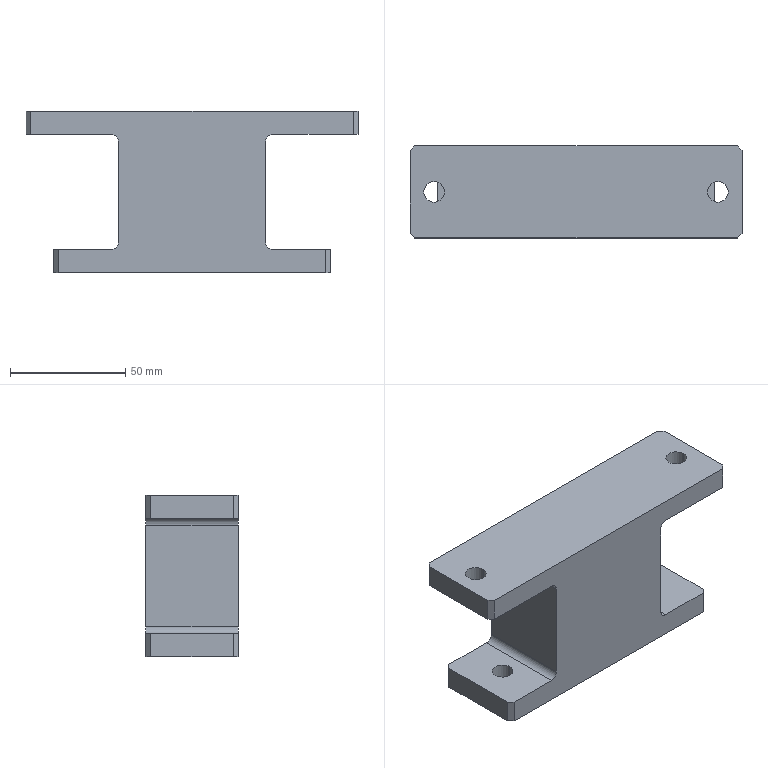Part | SolidWorks | features ICE 4, 3DProfileFeature 3, HoleWzd 3, Cut 2, Chamfer 1, Extrusion 1, Fillet 1, MirrorPattern 1 | 1 solid | 34 faces | box 144 x 40 x 70 mm | volume 231204 mm3 | plane 22 | cylinder 12 | commonest cylinder face diameters 9 x8 6 x4
STEP:
#1=CARTESIAN_POINT('',(78.784,24.549,10.));
#2=VERTEX_POINT('',#1);
#3=CARTESIAN_POINT('',(69.784,24.549,10.));
#4=VERTEX_POINT('',#3);
#5=CARTESIAN_POINT('',(74.284,24.549,10.));
#6=DIRECTION('',(0.,0.,-1.));
#7=DIRECTION('',(-1.,0.,0.));
#8=AXIS2_PLACEMENT_3D('',#5,#6,#7);
#9=CIRCLE('',#8,4.5);
#10=EDGE_CURVE('',#2,#4,#9,.T.);
#11=ORIENTED_EDGE('',*,*,#10,.F.);
#12=CARTESIAN_POINT('',(78.784,24.549,0.));
#13=VERTEX_POINT('',#12);
#14=CARTESIAN_POINT('',(78.784,24.549,0.));
#15=DIRECTION('',(0.,0.,-1.));
#16=VECTOR('',#15,1000.);
#17=LINE('',#14,#16);
#18=EDGE_CURVE('',#2,#13,#17,.T.);
#19=ORIENTED_EDGE('',*,*,#18,.T.);
#20=CARTESIAN_POINT('',(69.784,24.549,0.));
#21=VERTEX_POINT('',#20);
#22=CARTESIAN_POINT('',(74.284,24.549,0.));
#23=DIRECTION('',(0.,0.,-1.));
#24=DIRECTION('',(-1.,0.,0.));
#25=AXIS2_PLACEMENT_3D('',#22,#23,#24);
#26=CIRCLE('',#25,4.5);
#27=EDGE_CURVE('',#13,#21,#26,.T.);
#28=ORIENTED_EDGE('',*,*,#27,.T.);
#29=CARTESIAN_POINT('',(69.784,24.549,0.));
#30=DIRECTION('',(0.,0.,-1.));
#31=VECTOR('',#30,1000.);
#32=LINE('',#29,#31);
#33=EDGE_CURVE('',#4,#21,#32,.T.);
#34=ORIENTED_EDGE('',*,*,#33,.F.);
#35=EDGE_LOOP('',(#11,#19,#28,#34));
#36=FACE_OUTER_BOUND('',#35,.T.);
#37=CARTESIAN_POINT('',(74.284,24.549,0.));
#38=DIRECTION('',(0.,0.,-1.));
#39=DIRECTION('',(-1.,0.,0.));
#40=AXIS2_PLACEMENT_3D('',#37,#38,#39);
#41=CYLINDRICAL_SURFACE('',#40,4.5);
#42=ADVANCED_FACE('',(#36),#41,.F.);
#43=CARTESIAN_POINT('',(168.784,24.549,10.));
#44=VERTEX_POINT('',#43);
#45=CARTESIAN_POINT('',(159.784,24.549,10.));
#46=VERTEX_POINT('',#45);
#47=CARTESIAN_POINT('',(164.284,24.549,10.));
#48=DIRECTION('',(0.,0.,-1.));
#49=DIRECTION('',(-1.,0.,0.));
#50=AXIS2_PLACEMENT_3D('',#47,#48,#49);
#51=CIRCLE('',#50,4.5);
#52=EDGE_CURVE('',#44,#46,#51,.T.);
#53=ORIENTED_EDGE('',*,*,#52,.F.);
#54=CARTESIAN_POINT('',(168.784,24.549,0.));
#55=VERTEX_POINT('',#54);
#56=CARTESIAN_POINT('',(168.784,24.549,0.));
#57=DIRECTION('',(0.,0.,-1.));
#58=VECTOR('',#57,1000.);
#59=LINE('',#56,#58);
#60=EDGE_CURVE('',#44,#55,#59,.T.);
#61=ORIENTED_EDGE('',*,*,#60,.T.);
#62=CARTESIAN_POINT('',(159.784,24.549,0.));
#63=VERTEX_POINT('',#62);
#64=CARTESIAN_POINT('',(164.284,24.549,0.));
#65=DIRECTION('',(0.,0.,-1.));
#66=DIRECTION('',(-1.,0.,0.));
#67=AXIS2_PLACEMENT_3D('',#64,#65,#66);
#68=CIRCLE('',#67,4.5);
#69=EDGE_CURVE('',#55,#63,#68,.T.);
#70=ORIENTED_EDGE('',*,*,#69,.T.);
#71=CARTESIAN_POINT('',(159.784,24.549,0.));
#72=DIRECTION('',(0.,0.,-1.));
#73=VECTOR('',#72,1000.);
#74=LINE('',#71,#73);
#75=EDGE_CURVE('',#46,#63,#74,.T.);
#76=ORIENTED_EDGE('',*,*,#75,.F.);
#77=EDGE_LOOP('',(#53,#61,#70,#76));
#78=FACE_OUTER_BOUND('',#77,.T.);
#79=CARTESIAN_POINT('',(164.284,24.549,0.));
#80=DIRECTION('',(0.,0.,-1.));
#81=DIRECTION('',(-1.,0.,0.));
#82=AXIS2_PLACEMENT_3D('',#79,#80,#81);
#83=CYLINDRICAL_SURFACE('',#82,4.5);
#84=ADVANCED_FACE('',(#78),#83,.F.);
#85=CARTESIAN_POINT('',(176.284,24.549,60.));
#86=VERTEX_POINT('',#85);
#87=CARTESIAN_POINT('',(185.284,24.549,60.));
#88=VERTEX_POINT('',#87);
#89=CARTESIAN_POINT('',(180.784,24.549,60.));
#90=DIRECTION('',(0.,0.,1.));
#91=DIRECTION('',(1.,0.,0.));
#92=AXIS2_PLACEMENT_3D('',#89,#90,#91);
#93=CIRCLE('',#92,4.5);
#94=EDGE_CURVE('',#86,#88,#93,.T.);
#95=ORIENTED_EDGE('',*,*,#94,.F.);
#96=CARTESIAN_POINT('',(176.284,24.549,70.));
#97=VERTEX_POINT('',#96);
#98=CARTESIAN_POINT('',(176.284,24.549,47.272));
#99=DIRECTION('',(0.,0.,1.));
#100=VECTOR('',#99,1000.);
#101=LINE('',#98,#100);
#102=EDGE_CURVE('',#86,#97,#101,.T.);
#103=ORIENTED_EDGE('',*,*,#102,.T.);
#104=CARTESIAN_POINT('',(185.284,24.549,70.));
#105=VERTEX_POINT('',#104);
#106=CARTESIAN_POINT('',(180.784,24.549,70.));
#107=DIRECTION('',(0.,0.,-1.));
#108=DIRECTION('',(-1.,0.,0.));
#109=AXIS2_PLACEMENT_3D('',#106,#107,#108);
#110=CIRCLE('',#109,4.5);
#111=EDGE_CURVE('',#105,#97,#110,.T.);
#112=ORIENTED_EDGE('',*,*,#111,.F.);
#113=CARTESIAN_POINT('',(185.284,24.549,47.272));
#114=DIRECTION('',(0.,0.,1.));
#115=VECTOR('',#114,1000.);
#116=LINE('',#113,#115);
#117=EDGE_CURVE('',#88,#105,#116,.T.);
#118=ORIENTED_EDGE('',*,*,#117,.F.);
#119=EDGE_LOOP('',(#95,#103,#112,#118));
#120=FACE_OUTER_BOUND('',#119,.T.);
#121=CARTESIAN_POINT('',(180.784,24.549,47.272));
#122=DIRECTION('',(0.,0.,1.));
#123=DIRECTION('',(1.,0.,0.));
#124=AXIS2_PLACEMENT_3D('',#121,#122,#123);
#125=CYLINDRICAL_SURFACE('',#124,4.5);
#126=ADVANCED_FACE('',(#120),#125,.F.);
#127=CARTESIAN_POINT('',(62.284,24.549,60.));
#128=VERTEX_POINT('',#127);
#129=CARTESIAN_POINT('',(53.284,24.549,60.));
#130=VERTEX_POINT('',#129);
#131=CARTESIAN_POINT('',(57.784,24.549,60.));
#132=DIRECTION('',(0.,0.,-1.));
#133=DIRECTION('',(1.,0.,0.));
#134=AXIS2_PLACEMENT_3D('',#131,#132,#133);
#135=CIRCLE('',#134,4.5);
#136=EDGE_CURVE('',#128,#130,#135,.T.);
#137=ORIENTED_EDGE('',*,*,#136,.T.);
#138=CARTESIAN_POINT('',(53.284,24.549,70.));
#139=VERTEX_POINT('',#138);
#140=CARTESIAN_POINT('',(53.284,24.549,47.272));
#141=DIRECTION('',(0.,0.,1.));
#142=VECTOR('',#141,1000.);
#143=LINE('',#140,#142);
#144=EDGE_CURVE('',#130,#139,#143,.T.);
#145=ORIENTED_EDGE('',*,*,#144,.T.);
#146=CARTESIAN_POINT('',(62.284,24.549,70.));
#147=VERTEX_POINT('',#146);
#148=CARTESIAN_POINT('',(57.784,24.549,70.));
#149=DIRECTION('',(0.,0.,1.));
#150=DIRECTION('',(1.,0.,0.));
#151=AXIS2_PLACEMENT_3D('',#148,#149,#150);
#152=CIRCLE('',#151,4.5);
#153=EDGE_CURVE('',#139,#147,#152,.T.);
#154=ORIENTED_EDGE('',*,*,#153,.T.);
#155=CARTESIAN_POINT('',(62.284,24.549,47.272));
#156=DIRECTION('',(0.,0.,1.));
#157=VECTOR('',#156,1000.);
#158=LINE('',#155,#157);
#159=EDGE_CURVE('',#128,#147,#158,.T.);
#160=ORIENTED_EDGE('',*,*,#159,.F.);
#161=EDGE_LOOP('',(#137,#145,#154,#160));
#162=FACE_OUTER_BOUND('',#161,.T.);
#163=CARTESIAN_POINT('',(57.784,24.549,47.272));
#164=DIRECTION('',(0.,0.,1.));
#165=DIRECTION('',(1.,0.,0.));
#166=AXIS2_PLACEMENT_3D('',#163,#164,#165);
#167=CYLINDRICAL_SURFACE('',#166,4.5);
#168=ADVANCED_FACE('',(#162),#167,.F.);
#169=CARTESIAN_POINT('',(179.284,6.549,0.));
#170=VERTEX_POINT('',#169);
#171=CARTESIAN_POINT('',(179.284,42.549,0.));
#172=VERTEX_POINT('',#171);
#173=CARTESIAN_POINT('',(179.284,44.549,0.));
#174=DIRECTION('',(0.,1.,0.));
#175=VECTOR('',#174,1000.);
#176=LINE('',#173,#175);
#177=EDGE_CURVE('',#170,#172,#176,.T.);
#178=ORIENTED_EDGE('',*,*,#177,.T.);
#179=CARTESIAN_POINT('',(179.284,42.549,10.));
#180=VERTEX_POINT('',#179);
#181=CARTESIAN_POINT('',(179.284,42.549,70.));
#182=DIRECTION('',(0.,0.,1.));
#183=VECTOR('',#182,1000.);
#184=LINE('',#181,#183);
#185=EDGE_CURVE('',#172,#180,#184,.T.);
#186=ORIENTED_EDGE('',*,*,#185,.T.);
#187=CARTESIAN_POINT('',(179.284,6.549,10.));
#188=VERTEX_POINT('',#187);
#189=CARTESIAN_POINT('',(179.284,44.549,10.));
#190=DIRECTION('',(0.,-1.,0.));
#191=VECTOR('',#190,1000.);
#192=LINE('',#189,#191);
#193=EDGE_CURVE('',#180,#188,#192,.T.);
#194=ORIENTED_EDGE('',*,*,#193,.T.);
#195=CARTESIAN_POINT('',(179.284,6.549,70.));
#196=DIRECTION('',(0.,0.,-1.));
#197=VECTOR('',#196,1000.);
#198=LINE('',#195,#197);
#199=EDGE_CURVE('',#188,#170,#198,.T.);
#200=ORIENTED_EDGE('',*,*,#199,.T.);
#201=EDGE_LOOP('',(#178,#186,#194,#200));
#202=FACE_OUTER_BOUND('',#201,.T.);
#203=CARTESIAN_POINT('',(179.284,44.549,70.));
#204=DIRECTION('',(-1.,0.,0.));
#205=DIRECTION('',(0.,0.,1.));
#206=AXIS2_PLACEMENT_3D('',#203,#204,#205);
#207=PLANE('',#206);
#208=ADVANCED_FACE('',(#202),#207,.F.);
#209=CARTESIAN_POINT('',(177.284,44.549,0.));
#210=VERTEX_POINT('',#209);
#211=CARTESIAN_POINT('',(61.284,44.549,0.));
#212=VERTEX_POINT('',#211);
#213=CARTESIAN_POINT('',(179.284,44.549,0.));
#214=DIRECTION('',(-1.,0.,0.));
#215=VECTOR('',#214,1000.);
#216=LINE('',#213,#215);
#217=EDGE_CURVE('',#210,#212,#216,.T.);
#218=ORIENTED_EDGE('',*,*,#217,.T.);
#219=CARTESIAN_POINT('',(61.284,44.549,10.));
#220=VERTEX_POINT('',#219);
#221=CARTESIAN_POINT('',(61.284,44.549,70.));
#222=DIRECTION('',(0.,0.,1.));
#223=VECTOR('',#222,1000.);
#224=LINE('',#221,#223);
#225=EDGE_CURVE('',#212,#220,#224,.T.);
#226=ORIENTED_EDGE('',*,*,#225,.T.);
#227=CARTESIAN_POINT('',(84.284,44.549,10.));
#228=VERTEX_POINT('',#227);
#229=CARTESIAN_POINT('',(87.284,44.549,10.));
#230=DIRECTION('',(-1.,0.,0.));
#231=VECTOR('',#230,1000.);
#232=LINE('',#229,#231);
#233=EDGE_CURVE('',#228,#220,#232,.T.);
#234=ORIENTED_EDGE('',*,*,#233,.F.);
#235=CARTESIAN_POINT('',(87.284,44.549,13.));
#236=VERTEX_POINT('',#235);
#237=CARTESIAN_POINT('',(84.284,44.549,13.));
#238=DIRECTION('',(0.,-1.,0.));
#239=DIRECTION('',(0.,0.,-1.));
#240=AXIS2_PLACEMENT_3D('',#237,#238,#239);
#241=CIRCLE('',#240,3.);
#242=EDGE_CURVE('',#228,#236,#241,.T.);
#243=ORIENTED_EDGE('',*,*,#242,.T.);
#244=CARTESIAN_POINT('',(87.284,44.549,57.));
#245=VERTEX_POINT('',#244);
#246=CARTESIAN_POINT('',(87.284,44.549,60.));
#247=DIRECTION('',(0.,0.,-1.));
#248=VECTOR('',#247,1000.);
#249=LINE('',#246,#248);
#250=EDGE_CURVE('',#245,#236,#249,.T.);
#251=ORIENTED_EDGE('',*,*,#250,.F.);
#252=CARTESIAN_POINT('',(84.284,44.549,60.));
#253=VERTEX_POINT('',#252);
#254=CARTESIAN_POINT('',(84.284,44.549,57.));
#255=DIRECTION('',(0.,-1.,0.));
#256=DIRECTION('',(0.,0.,-1.));
#257=AXIS2_PLACEMENT_3D('',#254,#255,#256);
#258=CIRCLE('',#257,3.);
#259=EDGE_CURVE('',#245,#253,#258,.T.);
#260=ORIENTED_EDGE('',*,*,#259,.T.);
#261=CARTESIAN_POINT('',(49.284,44.549,60.));
#262=VERTEX_POINT('',#261);
#263=CARTESIAN_POINT('',(87.284,44.549,60.));
#264=DIRECTION('',(1.,0.,0.));
#265=VECTOR('',#264,1000.);
#266=LINE('',#263,#265);
#267=EDGE_CURVE('',#262,#253,#266,.T.);
#268=ORIENTED_EDGE('',*,*,#267,.F.);
#269=CARTESIAN_POINT('',(49.284,44.549,70.));
#270=VERTEX_POINT('',#269);
#271=CARTESIAN_POINT('',(49.284,44.549,70.));
#272=DIRECTION('',(0.,0.,1.));
#273=VECTOR('',#272,1000.);
#274=LINE('',#271,#273);
#275=EDGE_CURVE('',#262,#270,#274,.T.);
#276=ORIENTED_EDGE('',*,*,#275,.T.);
#277=CARTESIAN_POINT('',(189.284,44.549,70.));
#278=VERTEX_POINT('',#277);
#279=CARTESIAN_POINT('',(179.284,44.549,70.));
#280=DIRECTION('',(-1.,0.,0.));
#281=VECTOR('',#280,1000.);
#282=LINE('',#279,#281);
#283=EDGE_CURVE('',#278,#270,#282,.T.);
#284=ORIENTED_EDGE('',*,*,#283,.F.);
#285=CARTESIAN_POINT('',(189.284,44.549,60.));
#286=VERTEX_POINT('',#285);
#287=CARTESIAN_POINT('',(189.284,44.549,60.));
#288=DIRECTION('',(0.,0.,-1.));
#289=VECTOR('',#288,1000.);
#290=LINE('',#287,#289);
#291=EDGE_CURVE('',#278,#286,#290,.T.);
#292=ORIENTED_EDGE('',*,*,#291,.T.);
#293=CARTESIAN_POINT('',(154.284,44.549,60.));
#294=VERTEX_POINT('',#293);
#295=CARTESIAN_POINT('',(151.284,44.549,60.));
#296=DIRECTION('',(1.,0.,0.));
#297=VECTOR('',#296,1000.);
#298=LINE('',#295,#297);
#299=EDGE_CURVE('',#294,#286,#298,.T.);
#300=ORIENTED_EDGE('',*,*,#299,.F.);
#301=CARTESIAN_POINT('',(151.284,44.549,57.));
#302=VERTEX_POINT('',#301);
#303=CARTESIAN_POINT('',(154.284,44.549,57.));
#304=DIRECTION('',(0.,-1.,0.));
#305=DIRECTION('',(0.,0.,-1.));
#306=AXIS2_PLACEMENT_3D('',#303,#304,#305);
#307=CIRCLE('',#306,3.);
#308=EDGE_CURVE('',#294,#302,#307,.T.);
#309=ORIENTED_EDGE('',*,*,#308,.T.);
#310=CARTESIAN_POINT('',(151.284,44.549,13.));
#311=VERTEX_POINT('',#310);
#312=CARTESIAN_POINT('',(151.284,44.549,60.));
#313=DIRECTION('',(0.,0.,1.));
#314=VECTOR('',#313,1000.);
#315=LINE('',#312,#314);
#316=EDGE_CURVE('',#311,#302,#315,.T.);
#317=ORIENTED_EDGE('',*,*,#316,.F.);
#318=CARTESIAN_POINT('',(154.284,44.549,10.));
#319=VERTEX_POINT('',#318);
#320=CARTESIAN_POINT('',(154.284,44.549,13.));
#321=DIRECTION('',(0.,-1.,0.));
#322=DIRECTION('',(0.,0.,-1.));
#323=AXIS2_PLACEMENT_3D('',#320,#321,#322);
#324=CIRCLE('',#323,3.);
#325=EDGE_CURVE('',#311,#319,#324,.T.);
#326=ORIENTED_EDGE('',*,*,#325,.T.);
#327=CARTESIAN_POINT('',(177.284,44.549,10.));
#328=VERTEX_POINT('',#327);
#329=CARTESIAN_POINT('',(151.284,44.549,10.));
#330=DIRECTION('',(-1.,0.,0.));
#331=VECTOR('',#330,1000.);
#332=LINE('',#329,#331);
#333=EDGE_CURVE('',#328,#319,#332,.T.);
#334=ORIENTED_EDGE('',*,*,#333,.F.);
#335=CARTESIAN_POINT('',(177.284,44.549,70.));
#336=DIRECTION('',(0.,0.,-1.));
#337=VECTOR('',#336,1000.);
#338=LINE('',#335,#337);
#339=EDGE_CURVE('',#328,#210,#338,.T.);
#340=ORIENTED_EDGE('',*,*,#339,.T.);
#341=EDGE_LOOP('',(#218,#226,#234,#243,#251,#260,#268,#276,#284,#292,#300,#309,#317,#326,#334,#340));
#342=FACE_OUTER_BOUND('',#341,.T.);
#343=CARTESIAN_POINT('',(179.284,44.549,70.));
#344=DIRECTION('',(0.,-1.,0.));
#345=DIRECTION('',(0.,0.,-1.));
#346=AXIS2_PLACEMENT_3D('',#343,#344,#345);
#347=PLANE('',#346);
#348=ADVANCED_FACE('',(#342),#347,.F.);
#349=CARTESIAN_POINT('',(59.284,42.549,0.));
#350=VERTEX_POINT('',#349);
#351=CARTESIAN_POINT('',(59.284,6.549,0.));
#352=VERTEX_POINT('',#351);
#353=CARTESIAN_POINT('',(59.284,44.549,0.));
#354=DIRECTION('',(0.,-1.,0.));
#355=VECTOR('',#354,1000.);
#356=LINE('',#353,#355);
#357=EDGE_CURVE('',#350,#352,#356,.T.);
#358=ORIENTED_EDGE('',*,*,#357,.T.);
#359=CARTESIAN_POINT('',(59.284,6.549,10.));
#360=VERTEX_POINT('',#359);
#361=CARTESIAN_POINT('',(59.284,6.549,70.));
#362=DIRECTION('',(0.,0.,1.));
#363=VECTOR('',#362,1000.);
#364=LINE('',#361,#363);
#365=EDGE_CURVE('',#352,#360,#364,.T.);
#366=ORIENTED_EDGE('',*,*,#365,.T.);
#367=CARTESIAN_POINT('',(59.284,42.549,10.));
#368=VERTEX_POINT('',#367);
#369=CARTESIAN_POINT('',(59.284,44.549,10.));
#370=DIRECTION('',(0.,1.,0.));
#371=VECTOR('',#370,1000.);
#372=LINE('',#369,#371);
#373=EDGE_CURVE('',#360,#368,#372,.T.);
#374=ORIENTED_EDGE('',*,*,#373,.T.);
#375=CARTESIAN_POINT('',(59.284,42.549,70.));
#376=DIRECTION('',(0.,0.,-1.));
#377=VECTOR('',#376,1000.);
#378=LINE('',#375,#377);
#379=EDGE_CURVE('',#368,#350,#378,.T.);
#380=ORIENTED_EDGE('',*,*,#379,.T.);
#381=EDGE_LOOP('',(#358,#366,#374,#380));
#382=FACE_OUTER_BOUND('',#381,.T.);
#383=CARTESIAN_POINT('',(59.284,44.549,70.));
#384=DIRECTION('',(1.,0.,0.));
#385=DIRECTION('',(0.,0.,-1.));
#386=AXIS2_PLACEMENT_3D('',#383,#384,#385);
#387=PLANE('',#386);
#388=ADVANCED_FACE('',(#382),#387,.F.);
#389=CARTESIAN_POINT('',(84.284,4.549,10.));
#390=VERTEX_POINT('',#389);
#391=CARTESIAN_POINT('',(61.284,4.549,10.));
#392=VERTEX_POINT('',#391);
#393=CARTESIAN_POINT('',(87.284,4.549,10.));
#394=DIRECTION('',(-1.,0.,0.));
#395=VECTOR('',#394,1000.);
#396=LINE('',#393,#395);
#397=EDGE_CURVE('',#390,#392,#396,.T.);
#398=ORIENTED_EDGE('',*,*,#397,.T.);
#399=CARTESIAN_POINT('',(61.284,4.549,0.));
#400=VERTEX_POINT('',#399);
#401=CARTESIAN_POINT('',(61.284,4.549,70.));
#402=DIRECTION('',(0.,0.,-1.));
#403=VECTOR('',#402,1000.);
#404=LINE('',#401,#403);
#405=EDGE_CURVE('',#392,#400,#404,.T.);
#406=ORIENTED_EDGE('',*,*,#405,.T.);
#407=CARTESIAN_POINT('',(177.284,4.549,0.));
#408=VERTEX_POINT('',#407);
#409=CARTESIAN_POINT('',(179.284,4.549,0.));
#410=DIRECTION('',(1.,0.,0.));
#411=VECTOR('',#410,1000.);
#412=LINE('',#409,#411);
#413=EDGE_CURVE('',#400,#408,#412,.T.);
#414=ORIENTED_EDGE('',*,*,#413,.T.);
#415=CARTESIAN_POINT('',(177.284,4.549,10.));
#416=VERTEX_POINT('',#415);
#417=CARTESIAN_POINT('',(177.284,4.549,70.));
#418=DIRECTION('',(0.,0.,1.));
#419=VECTOR('',#418,1000.);
#420=LINE('',#417,#419);
#421=EDGE_CURVE('',#408,#416,#420,.T.);
#422=ORIENTED_EDGE('',*,*,#421,.T.);
#423=CARTESIAN_POINT('',(154.284,4.549,10.));
#424=VERTEX_POINT('',#423);
#425=CARTESIAN_POINT('',(151.284,4.549,10.));
#426=DIRECTION('',(-1.,0.,0.));
#427=VECTOR('',#426,1000.);
#428=LINE('',#425,#427);
#429=EDGE_CURVE('',#416,#424,#428,.T.);
#430=ORIENTED_EDGE('',*,*,#429,.T.);
#431=CARTESIAN_POINT('',(151.284,4.549,13.));
#432=VERTEX_POINT('',#431);
#433=CARTESIAN_POINT('',(154.284,4.549,13.));
#434=DIRECTION('',(0.,1.,0.));
#435=DIRECTION('',(-1.,0.,0.));
#436=AXIS2_PLACEMENT_3D('',#433,#434,#435);
#437=CIRCLE('',#436,3.);
#438=EDGE_CURVE('',#424,#432,#437,.T.);
#439=ORIENTED_EDGE('',*,*,#438,.T.);
#440=CARTESIAN_POINT('',(151.284,4.549,57.));
#441=VERTEX_POINT('',#440);
#442=CARTESIAN_POINT('',(151.284,4.549,60.));
#443=DIRECTION('',(0.,0.,1.));
#444=VECTOR('',#443,1000.);
#445=LINE('',#442,#444);
#446=EDGE_CURVE('',#432,#441,#445,.T.);
#447=ORIENTED_EDGE('',*,*,#446,.T.);
#448=CARTESIAN_POINT('',(154.284,4.549,60.));
#449=VERTEX_POINT('',#448);
#450=CARTESIAN_POINT('',(154.284,4.549,57.));
#451=DIRECTION('',(0.,1.,0.));
#452=DIRECTION('',(-1.,0.,0.));
#453=AXIS2_PLACEMENT_3D('',#450,#451,#452);
#454=CIRCLE('',#453,3.);
#455=EDGE_CURVE('',#441,#449,#454,.T.);
#456=ORIENTED_EDGE('',*,*,#455,.T.);
#457=CARTESIAN_POINT('',(189.284,4.549,60.));
#458=VERTEX_POINT('',#457);
#459=CARTESIAN_POINT('',(151.284,4.549,60.));
#460=DIRECTION('',(1.,0.,0.));
#461=VECTOR('',#460,1000.);
#462=LINE('',#459,#461);
#463=EDGE_CURVE('',#449,#458,#462,.T.);
#464=ORIENTED_EDGE('',*,*,#463,.T.);
#465=CARTESIAN_POINT('',(189.284,4.549,70.));
#466=VERTEX_POINT('',#465);
#467=CARTESIAN_POINT('',(189.284,4.549,70.));
#468=DIRECTION('',(0.,0.,1.));
#469=VECTOR('',#468,1000.);
#470=LINE('',#467,#469);
#471=EDGE_CURVE('',#458,#466,#470,.T.);
#472=ORIENTED_EDGE('',*,*,#471,.T.);
#473=CARTESIAN_POINT('',(49.284,4.549,70.));
#474=VERTEX_POINT('',#473);
#475=CARTESIAN_POINT('',(179.284,4.549,70.));
#476=DIRECTION('',(1.,0.,0.));
#477=VECTOR('',#476,1000.);
#478=LINE('',#475,#477);
#479=EDGE_CURVE('',#474,#466,#478,.T.);
#480=ORIENTED_EDGE('',*,*,#479,.F.);
#481=CARTESIAN_POINT('',(49.284,4.549,60.));
#482=VERTEX_POINT('',#481);
#483=CARTESIAN_POINT('',(49.284,4.549,60.));
#484=DIRECTION('',(0.,0.,-1.));
#485=VECTOR('',#484,1000.);
#486=LINE('',#483,#485);
#487=EDGE_CURVE('',#474,#482,#486,.T.);
#488=ORIENTED_EDGE('',*,*,#487,.T.);
#489=CARTESIAN_POINT('',(84.284,4.549,60.));
#490=VERTEX_POINT('',#489);
#491=CARTESIAN_POINT('',(87.284,4.549,60.));
#492=DIRECTION('',(1.,0.,0.));
#493=VECTOR('',#492,1000.);
#494=LINE('',#491,#493);
#495=EDGE_CURVE('',#482,#490,#494,.T.);
#496=ORIENTED_EDGE('',*,*,#495,.T.);
#497=CARTESIAN_POINT('',(87.284,4.549,57.));
#498=VERTEX_POINT('',#497);
#499=CARTESIAN_POINT('',(84.284,4.549,57.));
#500=DIRECTION('',(0.,1.,0.));
#501=DIRECTION('',(-1.,0.,0.));
#502=AXIS2_PLACEMENT_3D('',#499,#500,#501);
#503=CIRCLE('',#502,3.);
#504=EDGE_CURVE('',#490,#498,#503,.T.);
#505=ORIENTED_EDGE('',*,*,#504,.T.);
#506=CARTESIAN_POINT('',(87.284,4.549,13.));
#507=VERTEX_POINT('',#506);
#508=CARTESIAN_POINT('',(87.284,4.549,60.));
#509=DIRECTION('',(0.,0.,-1.));
#510=VECTOR('',#509,1000.);
#511=LINE('',#508,#510);
#512=EDGE_CURVE('',#498,#507,#511,.T.);
#513=ORIENTED_EDGE('',*,*,#512,.T.);
#514=CARTESIAN_POINT('',(84.284,4.549,13.));
#515=DIRECTION('',(0.,1.,0.));
#516=DIRECTION('',(-1.,0.,0.));
#517=AXIS2_PLACEMENT_3D('',#514,#515,#516);
#518=CIRCLE('',#517,3.);
#519=EDGE_CURVE('',#507,#390,#518,.T.);
#520=ORIENTED_EDGE('',*,*,#519,.T.);
#521=EDGE_LOOP('',(#398,#406,#414,#422,#430,#439,#447,#456,#464,#472,#480,#488,#496,#505,#513,#520));
#522=FACE_OUTER_BOUND('',#521,.T.);
#523=CARTESIAN_POINT('',(179.284,4.549,70.));
#524=DIRECTION('',(0.,1.,0.));
#525=DIRECTION('',(-1.,0.,0.));
#526=AXIS2_PLACEMENT_3D('',#523,#524,#525);
#527=PLANE('',#526);
#528=ADVANCED_FACE('',(#522),#527,.F.);
#529=ORIENTED_EDGE('',*,*,#111,.T.);
#530=CARTESIAN_POINT('',(180.784,24.549,70.));
#531=DIRECTION('',(0.,0.,-1.));
#532=DIRECTION('',(-1.,0.,0.));
#533=AXIS2_PLACEMENT_3D('',#530,#531,#532);
#534=CIRCLE('',#533,4.5);
#535=EDGE_CURVE('',#97,#105,#534,.T.);
#536=ORIENTED_EDGE('',*,*,#535,.T.);
#537=EDGE_LOOP('',(#529,#536));
#538=FACE_BOUND('',#537,.T.);
#539=CARTESIAN_POINT('',(57.784,24.549,70.));
#540=DIRECTION('',(0.,0.,1.));
#541=DIRECTION('',(1.,0.,0.));
#542=AXIS2_PLACEMENT_3D('',#539,#540,#541);
#543=CIRCLE('',#542,4.5);
#544=EDGE_CURVE('',#147,#139,#543,.T.);
#545=ORIENTED_EDGE('',*,*,#544,.F.);
#546=ORIENTED_EDGE('',*,*,#153,.F.);
#547=EDGE_LOOP('',(#545,#546));
#548=FACE_BOUND('',#547,.T.);
#549=ORIENTED_EDGE('',*,*,#479,.T.);
#550=CARTESIAN_POINT('',(191.284,6.549,70.));
#551=VERTEX_POINT('',#550);
#552=CARTESIAN_POINT('',(191.284,6.549,70.));
#553=DIRECTION('',(0.7071,0.7071,0.));
#554=VECTOR('',#553,1000.);
#555=LINE('',#552,#554);
#556=EDGE_CURVE('',#466,#551,#555,.T.);
#557=ORIENTED_EDGE('',*,*,#556,.T.);
#558=CARTESIAN_POINT('',(191.284,42.549,70.));
#559=VERTEX_POINT('',#558);
#560=CARTESIAN_POINT('',(191.284,4.549,70.));
#561=DIRECTION('',(0.,-1.,0.));
#562=VECTOR('',#561,1000.);
#563=LINE('',#560,#562);
#564=EDGE_CURVE('',#559,#551,#563,.T.);
#565=ORIENTED_EDGE('',*,*,#564,.F.);
#566=CARTESIAN_POINT('',(189.284,44.549,70.));
#567=DIRECTION('',(-0.7071,0.7071,0.));
#568=VECTOR('',#567,1000.);
#569=LINE('',#566,#568);
#570=EDGE_CURVE('',#559,#278,#569,.T.);
#571=ORIENTED_EDGE('',*,*,#570,.T.);
#572=ORIENTED_EDGE('',*,*,#283,.T.);
#573=CARTESIAN_POINT('',(47.284,42.549,70.));
#574=VERTEX_POINT('',#573);
#575=CARTESIAN_POINT('',(49.284,44.549,70.));
#576=DIRECTION('',(-0.7071,-0.7071,0.));
#577=VECTOR('',#576,1000.);
#578=LINE('',#575,#577);
#579=EDGE_CURVE('',#270,#574,#578,.T.);
#580=ORIENTED_EDGE('',*,*,#579,.T.);
#581=CARTESIAN_POINT('',(47.284,6.549,70.));
#582=VERTEX_POINT('',#581);
#583=CARTESIAN_POINT('',(47.284,44.549,70.));
#584=DIRECTION('',(0.,-1.,0.));
#585=VECTOR('',#584,1000.);
#586=LINE('',#583,#585);
#587=EDGE_CURVE('',#574,#582,#586,.T.);
#588=ORIENTED_EDGE('',*,*,#587,.T.);
#589=CARTESIAN_POINT('',(47.284,6.549,70.));
#590=DIRECTION('',(0.7071,-0.7071,0.));
#591=VECTOR('',#590,1000.);
#592=LINE('',#589,#591);
#593=EDGE_CURVE('',#582,#474,#592,.T.);
#594=ORIENTED_EDGE('',*,*,#593,.T.);
#595=EDGE_LOOP('',(#549,#557,#565,#571,#572,#580,#588,#594));
#596=FACE_OUTER_BOUND('',#595,.T.);
#597=CARTESIAN_POINT('',(0.,0.,70.));
#598=DIRECTION('',(0.,0.,-1.));
#599=DIRECTION('',(-1.,0.,0.));
#600=AXIS2_PLACEMENT_3D('',#597,#598,#599);
#601=PLANE('',#600);
#602=ADVANCED_FACE('',(#538,#548,#596),#601,.F.);
#603=CARTESIAN_POINT('',(74.284,24.549,0.));
#604=DIRECTION('',(0.,0.,-1.));
#605=DIRECTION('',(-1.,0.,0.));
#606=AXIS2_PLACEMENT_3D('',#603,#604,#605);
#607=CIRCLE('',#606,4.5);
#608=EDGE_CURVE('',#21,#13,#607,.T.);
#609=ORIENTED_EDGE('',*,*,#608,.F.);
#610=ORIENTED_EDGE('',*,*,#27,.F.);
#611=EDGE_LOOP('',(#609,#610));
#612=FACE_BOUND('',#611,.T.);
#613=CARTESIAN_POINT('',(164.284,24.549,0.));
#614=DIRECTION('',(0.,0.,-1.));
#615=DIRECTION('',(-1.,0.,0.));
#616=AXIS2_PLACEMENT_3D('',#613,#614,#615);
#617=CIRCLE('',#616,4.5);
#618=EDGE_CURVE('',#63,#55,#617,.T.);
#619=ORIENTED_EDGE('',*,*,#618,.F.);
#620=ORIENTED_EDGE('',*,*,#69,.F.);
#621=EDGE_LOOP('',(#619,#620));
#622=FACE_BOUND('',#621,.T.);
#623=ORIENTED_EDGE('',*,*,#413,.F.);
#624=CARTESIAN_POINT('',(32.917,32.917,0.));
#625=DIRECTION('',(-0.7071,0.7071,0.));
#626=VECTOR('',#625,1000.);
#627=LINE('',#624,#626);
#628=EDGE_CURVE('',#400,#352,#627,.T.);
#629=ORIENTED_EDGE('',*,*,#628,.T.);
#630=ORIENTED_EDGE('',*,*,#357,.F.);
#631=CARTESIAN_POINT('',(8.368,-8.368,0.));
#632=DIRECTION('',(0.7071,0.7071,0.));
#633=VECTOR('',#632,1000.);
#634=LINE('',#631,#633);
#635=EDGE_CURVE('',#350,#212,#634,.T.);
#636=ORIENTED_EDGE('',*,*,#635,.T.);
#637=ORIENTED_EDGE('',*,*,#217,.F.);
#638=CARTESIAN_POINT('',(110.917,110.917,0.));
#639=DIRECTION('',(0.7071,-0.7071,0.));
#640=VECTOR('',#639,1000.);
#641=LINE('',#638,#640);
#642=EDGE_CURVE('',#210,#172,#641,.T.);
#643=ORIENTED_EDGE('',*,*,#642,.T.);
#644=ORIENTED_EDGE('',*,*,#177,.F.);
#645=CARTESIAN_POINT('',(86.368,-86.368,0.));
#646=DIRECTION('',(-0.7071,-0.7071,0.));
#647=VECTOR('',#646,1000.);
#648=LINE('',#645,#647);
#649=EDGE_CURVE('',#170,#408,#648,.T.);
#650=ORIENTED_EDGE('',*,*,#649,.T.);
#651=EDGE_LOOP('',(#623,#629,#630,#636,#637,#643,#644,#650));
#652=FACE_OUTER_BOUND('',#651,.T.);
#653=CARTESIAN_POINT('',(0.,0.,0.));
#654=DIRECTION('',(0.,0.,-1.));
#655=DIRECTION('',(-1.,0.,0.));
#656=AXIS2_PLACEMENT_3D('',#653,#654,#655);
#657=PLANE('',#656);
#658=ADVANCED_FACE('',(#612,#622,#652),#657,.T.);
#659=CARTESIAN_POINT('',(164.284,24.549,10.));
#660=DIRECTION('',(0.,0.,-1.));
#661=DIRECTION('',(-1.,0.,0.));
#662=AXIS2_PLACEMENT_3D('',#659,#660,#661);
#663=CIRCLE('',#662,4.5);
#664=EDGE_CURVE('',#46,#44,#663,.T.);
#665=ORIENTED_EDGE('',*,*,#664,.T.);
#666=ORIENTED_EDGE('',*,*,#52,.T.);
#667=EDGE_LOOP('',(#665,#666));
#668=FACE_BOUND('',#667,.T.);
#669=ORIENTED_EDGE('',*,*,#193,.F.);
#670=CARTESIAN_POINT('',(177.284,44.549,10.));
#671=DIRECTION('',(-0.7071,0.7071,0.));
#672=VECTOR('',#671,1000.);
#673=LINE('',#670,#672);
#674=EDGE_CURVE('',#180,#328,#673,.T.);
#675=ORIENTED_EDGE('',*,*,#674,.T.);
#676=ORIENTED_EDGE('',*,*,#333,.T.);
#677=CARTESIAN_POINT('',(154.284,4.549,10.));
#678=DIRECTION('',(0.,-1.,0.));
#679=VECTOR('',#678,1000.);
#680=LINE('',#677,#679);
#681=EDGE_CURVE('',#319,#424,#680,.T.);
#682=ORIENTED_EDGE('',*,*,#681,.T.);
#683=ORIENTED_EDGE('',*,*,#429,.F.);
#684=CARTESIAN_POINT('',(179.284,6.549,10.));
#685=DIRECTION('',(0.7071,0.7071,0.));
#686=VECTOR('',#685,1000.);
#687=LINE('',#684,#686);
#688=EDGE_CURVE('',#416,#188,#687,.T.);
#689=ORIENTED_EDGE('',*,*,#688,.T.);
#690=EDGE_LOOP('',(#669,#675,#676,#682,#683,#689));
#691=FACE_OUTER_BOUND('',#690,.T.);
#692=CARTESIAN_POINT('',(151.284,4.549,10.));
#693=DIRECTION('',(0.,0.,-1.));
#694=DIRECTION('',(-1.,0.,0.));
#695=AXIS2_PLACEMENT_3D('',#692,#693,#694);
#696=PLANE('',#695);
#697=ADVANCED_FACE('',(#668,#691),#696,.F.);
#698=CARTESIAN_POINT('',(180.784,24.549,60.));
#699=DIRECTION('',(0.,0.,1.));
#700=DIRECTION('',(1.,0.,0.));
#701=AXIS2_PLACEMENT_3D('',#698,#699,#700);
#702=CIRCLE('',#701,4.5);
#703=EDGE_CURVE('',#88,#86,#702,.T.);
#704=ORIENTED_EDGE('',*,*,#703,.T.);
#705=ORIENTED_EDGE('',*,*,#94,.T.);
#706=EDGE_LOOP('',(#704,#705));
#707=FACE_BOUND('',#706,.T.);
#708=CARTESIAN_POINT('',(191.284,42.549,60.));
#709=VERTEX_POINT('',#708);
#710=CARTESIAN_POINT('',(191.284,6.549,60.));
#711=VERTEX_POINT('',#710);
#712=CARTESIAN_POINT('',(191.284,4.549,60.));
#713=DIRECTION('',(0.,-1.,0.));
#714=VECTOR('',#713,1000.);
#715=LINE('',#712,#714);
#716=EDGE_CURVE('',#709,#711,#715,.T.);
#717=ORIENTED_EDGE('',*,*,#716,.T.);
#718=CARTESIAN_POINT('',(191.284,6.549,60.));
#719=DIRECTION('',(-0.7071,-0.7071,0.));
#720=VECTOR('',#719,1000.);
#721=LINE('',#718,#720);
#722=EDGE_CURVE('',#711,#458,#721,.T.);
#723=ORIENTED_EDGE('',*,*,#722,.T.);
#724=ORIENTED_EDGE('',*,*,#463,.F.);
#725=CARTESIAN_POINT('',(154.284,44.549,60.));
#726=DIRECTION('',(0.,1.,0.));
#727=VECTOR('',#726,1000.);
#728=LINE('',#725,#727);
#729=EDGE_CURVE('',#449,#294,#728,.T.);
#730=ORIENTED_EDGE('',*,*,#729,.T.);
#731=ORIENTED_EDGE('',*,*,#299,.T.);
#732=CARTESIAN_POINT('',(189.284,44.549,60.));
#733=DIRECTION('',(0.7071,-0.7071,0.));
#734=VECTOR('',#733,1000.);
#735=LINE('',#732,#734);
#736=EDGE_CURVE('',#286,#709,#735,.T.);
#737=ORIENTED_EDGE('',*,*,#736,.T.);
#738=EDGE_LOOP('',(#717,#723,#724,#730,#731,#737));
#739=FACE_OUTER_BOUND('',#738,.T.);
#740=CARTESIAN_POINT('',(151.284,4.549,60.));
#741=DIRECTION('',(0.,0.,1.));
#742=DIRECTION('',(1.,0.,0.));
#743=AXIS2_PLACEMENT_3D('',#740,#741,#742);
#744=PLANE('',#743);
#745=ADVANCED_FACE('',(#707,#739),#744,.F.);
#746=ORIENTED_EDGE('',*,*,#446,.F.);
#747=CARTESIAN_POINT('',(151.284,44.549,13.));
#748=DIRECTION('',(0.,1.,0.));
#749=VECTOR('',#748,1000.);
#750=LINE('',#747,#749);
#751=EDGE_CURVE('',#432,#311,#750,.T.);
#752=ORIENTED_EDGE('',*,*,#751,.T.);
#753=ORIENTED_EDGE('',*,*,#316,.T.);
#754=CARTESIAN_POINT('',(151.284,4.549,57.));
#755=DIRECTION('',(0.,-1.,0.));
#756=VECTOR('',#755,1000.);
#757=LINE('',#754,#756);
#758=EDGE_CURVE('',#302,#441,#757,.T.);
#759=ORIENTED_EDGE('',*,*,#758,.T.);
#760=EDGE_LOOP('',(#746,#752,#753,#759));
#761=FACE_OUTER_BOUND('',#760,.T.);
#762=CARTESIAN_POINT('',(151.284,4.549,60.));
#763=DIRECTION('',(-1.,0.,0.));
#764=DIRECTION('',(0.,0.,1.));
#765=AXIS2_PLACEMENT_3D('',#762,#763,#764);
#766=PLANE('',#765);
#767=ADVANCED_FACE('',(#761),#766,.F.);
#768=ORIENTED_EDGE('',*,*,#136,.F.);
#769=CARTESIAN_POINT('',(57.784,24.549,60.));
#770=DIRECTION('',(0.,0.,-1.));
#771=DIRECTION('',(1.,0.,0.));
#772=AXIS2_PLACEMENT_3D('',#769,#770,#771);
#773=CIRCLE('',#772,4.5);
#774=EDGE_CURVE('',#130,#128,#773,.T.);
#775=ORIENTED_EDGE('',*,*,#774,.F.);
#776=EDGE_LOOP('',(#768,#775));
#777=FACE_BOUND('',#776,.T.);
#778=ORIENTED_EDGE('',*,*,#495,.F.);
#779=CARTESIAN_POINT('',(47.284,6.549,60.));
#780=VERTEX_POINT('',#779);
#781=CARTESIAN_POINT('',(47.284,6.549,60.));
#782=DIRECTION('',(-0.7071,0.7071,0.));
#783=VECTOR('',#782,1000.);
#784=LINE('',#781,#783);
#785=EDGE_CURVE('',#482,#780,#784,.T.);
#786=ORIENTED_EDGE('',*,*,#785,.T.);
#787=CARTESIAN_POINT('',(47.284,42.549,60.));
#788=VERTEX_POINT('',#787);
#789=CARTESIAN_POINT('',(47.284,44.549,60.));
#790=DIRECTION('',(0.,1.,0.));
#791=VECTOR('',#790,1000.);
#792=LINE('',#789,#791);
#793=EDGE_CURVE('',#780,#788,#792,.T.);
#794=ORIENTED_EDGE('',*,*,#793,.T.);
#795=CARTESIAN_POINT('',(49.284,44.549,60.));
#796=DIRECTION('',(0.7071,0.7071,0.));
#797=VECTOR('',#796,1000.);
#798=LINE('',#795,#797);
#799=EDGE_CURVE('',#788,#262,#798,.T.);
#800=ORIENTED_EDGE('',*,*,#799,.T.);
#801=ORIENTED_EDGE('',*,*,#267,.T.);
#802=CARTESIAN_POINT('',(84.284,4.549,60.));
#803=DIRECTION('',(0.,-1.,0.));
#804=VECTOR('',#803,1000.);
#805=LINE('',#802,#804);
#806=EDGE_CURVE('',#253,#490,#805,.T.);
#807=ORIENTED_EDGE('',*,*,#806,.T.);
#808=EDGE_LOOP('',(#778,#786,#794,#800,#801,#807));
#809=FACE_OUTER_BOUND('',#808,.T.);
#810=CARTESIAN_POINT('',(87.284,4.549,60.));
#811=DIRECTION('',(0.,0.,1.));
#812=DIRECTION('',(1.,0.,0.));
#813=AXIS2_PLACEMENT_3D('',#810,#811,#812);
#814=PLANE('',#813);
#815=ADVANCED_FACE('',(#777,#809),#814,.F.);
#816=CARTESIAN_POINT('',(74.284,24.549,10.));
#817=DIRECTION('',(0.,0.,-1.));
#818=DIRECTION('',(-1.,0.,0.));
#819=AXIS2_PLACEMENT_3D('',#816,#817,#818);
#820=CIRCLE('',#819,4.5);
#821=EDGE_CURVE('',#4,#2,#820,.T.);
#822=ORIENTED_EDGE('',*,*,#821,.T.);
#823=ORIENTED_EDGE('',*,*,#10,.T.);
#824=EDGE_LOOP('',(#822,#823));
#825=FACE_BOUND('',#824,.T.);
#826=ORIENTED_EDGE('',*,*,#373,.F.);
#827=CARTESIAN_POINT('',(61.284,4.549,10.));
#828=DIRECTION('',(0.7071,-0.7071,0.));
#829=VECTOR('',#828,1000.);
#830=LINE('',#827,#829);
#831=EDGE_CURVE('',#360,#392,#830,.T.);
#832=ORIENTED_EDGE('',*,*,#831,.T.);
#833=ORIENTED_EDGE('',*,*,#397,.F.);
#834=CARTESIAN_POINT('',(84.284,44.549,10.));
#835=DIRECTION('',(0.,1.,0.));
#836=VECTOR('',#835,1000.);
#837=LINE('',#834,#836);
#838=EDGE_CURVE('',#390,#228,#837,.T.);
#839=ORIENTED_EDGE('',*,*,#838,.T.);
#840=ORIENTED_EDGE('',*,*,#233,.T.);
#841=CARTESIAN_POINT('',(59.284,42.549,10.));
#842=DIRECTION('',(-0.7071,-0.7071,0.));
#843=VECTOR('',#842,1000.);
#844=LINE('',#841,#843);
#845=EDGE_CURVE('',#220,#368,#844,.T.);
#846=ORIENTED_EDGE('',*,*,#845,.T.);
#847=EDGE_LOOP('',(#826,#832,#833,#839,#840,#846));
#848=FACE_OUTER_BOUND('',#847,.T.);
#849=CARTESIAN_POINT('',(87.284,4.549,10.));
#850=DIRECTION('',(0.,0.,-1.));
#851=DIRECTION('',(-1.,0.,0.));
#852=AXIS2_PLACEMENT_3D('',#849,#850,#851);
#853=PLANE('',#852);
#854=ADVANCED_FACE('',(#825,#848),#853,.F.);
#855=ORIENTED_EDGE('',*,*,#250,.T.);
#856=CARTESIAN_POINT('',(87.284,4.549,13.));
#857=DIRECTION('',(0.,-1.,0.));
#858=VECTOR('',#857,1000.);
#859=LINE('',#856,#858);
#860=EDGE_CURVE('',#236,#507,#859,.T.);
#861=ORIENTED_EDGE('',*,*,#860,.T.);
#862=ORIENTED_EDGE('',*,*,#512,.F.);
#863=CARTESIAN_POINT('',(87.284,44.549,57.));
#864=DIRECTION('',(0.,1.,0.));
#865=VECTOR('',#864,1000.);
#866=LINE('',#863,#865);
#867=EDGE_CURVE('',#498,#245,#866,.T.);
#868=ORIENTED_EDGE('',*,*,#867,.T.);
#869=EDGE_LOOP('',(#855,#861,#862,#868));
#870=FACE_OUTER_BOUND('',#869,.T.);
#871=CARTESIAN_POINT('',(87.284,4.549,60.));
#872=DIRECTION('',(1.,0.,0.));
#873=DIRECTION('',(0.,0.,-1.));
#874=AXIS2_PLACEMENT_3D('',#871,#872,#873);
#875=PLANE('',#874);
#876=ADVANCED_FACE('',(#870),#875,.F.);
#877=ORIENTED_EDGE('',*,*,#519,.F.);
#878=ORIENTED_EDGE('',*,*,#860,.F.);
#879=ORIENTED_EDGE('',*,*,#242,.F.);
#880=ORIENTED_EDGE('',*,*,#838,.F.);
#881=EDGE_LOOP('',(#877,#878,#879,#880));
#882=FACE_OUTER_BOUND('',#881,.T.);
#883=CARTESIAN_POINT('',(84.284,4.549,13.));
#884=DIRECTION('',(0.,-1.,0.));
#885=DIRECTION('',(0.,0.,-1.));
#886=AXIS2_PLACEMENT_3D('',#883,#884,#885);
#887=CYLINDRICAL_SURFACE('',#886,3.);
#888=ADVANCED_FACE('',(#882),#887,.F.);
#889=ORIENTED_EDGE('',*,*,#438,.F.);
#890=ORIENTED_EDGE('',*,*,#681,.F.);
#891=ORIENTED_EDGE('',*,*,#325,.F.);
#892=ORIENTED_EDGE('',*,*,#751,.F.);
#893=EDGE_LOOP('',(#889,#890,#891,#892));
#894=FACE_OUTER_BOUND('',#893,.T.);
#895=CARTESIAN_POINT('',(154.284,4.549,13.));
#896=DIRECTION('',(0.,-1.,0.));
#897=DIRECTION('',(0.,0.,-1.));
#898=AXIS2_PLACEMENT_3D('',#895,#896,#897);
#899=CYLINDRICAL_SURFACE('',#898,3.);
#900=ADVANCED_FACE('',(#894),#899,.F.);
#901=ORIENTED_EDGE('',*,*,#504,.F.);
#902=ORIENTED_EDGE('',*,*,#806,.F.);
#903=ORIENTED_EDGE('',*,*,#259,.F.);
#904=ORIENTED_EDGE('',*,*,#867,.F.);
#905=EDGE_LOOP('',(#901,#902,#903,#904));
#906=FACE_OUTER_BOUND('',#905,.T.);
#907=CARTESIAN_POINT('',(84.284,4.549,57.));
#908=DIRECTION('',(0.,-1.,0.));
#909=DIRECTION('',(0.,0.,-1.));
#910=AXIS2_PLACEMENT_3D('',#907,#908,#909);
#911=CYLINDRICAL_SURFACE('',#910,3.);
#912=ADVANCED_FACE('',(#906),#911,.F.);
#913=ORIENTED_EDGE('',*,*,#455,.F.);
#914=ORIENTED_EDGE('',*,*,#758,.F.);
#915=ORIENTED_EDGE('',*,*,#308,.F.);
#916=ORIENTED_EDGE('',*,*,#729,.F.);
#917=EDGE_LOOP('',(#913,#914,#915,#916));
#918=FACE_OUTER_BOUND('',#917,.T.);
#919=CARTESIAN_POINT('',(154.284,4.549,57.));
#920=DIRECTION('',(0.,-1.,0.));
#921=DIRECTION('',(0.,0.,-1.));
#922=AXIS2_PLACEMENT_3D('',#919,#920,#921);
#923=CYLINDRICAL_SURFACE('',#922,3.);
#924=ADVANCED_FACE('',(#918),#923,.F.);
#925=ORIENTED_EDGE('',*,*,#564,.T.);
#926=CARTESIAN_POINT('',(191.284,6.549,60.));
#927=DIRECTION('',(0.,0.,-1.));
#928=VECTOR('',#927,1000.);
#929=LINE('',#926,#928);
#930=EDGE_CURVE('',#551,#711,#929,.T.);
#931=ORIENTED_EDGE('',*,*,#930,.T.);
#932=ORIENTED_EDGE('',*,*,#716,.F.);
#933=CARTESIAN_POINT('',(191.284,42.549,70.));
#934=DIRECTION('',(0.,0.,1.));
#935=VECTOR('',#934,1000.);
#936=LINE('',#933,#935);
#937=EDGE_CURVE('',#709,#559,#936,.T.);
#938=ORIENTED_EDGE('',*,*,#937,.T.);
#939=EDGE_LOOP('',(#925,#931,#932,#938));
#940=FACE_OUTER_BOUND('',#939,.T.);
#941=CARTESIAN_POINT('',(191.284,4.549,70.));
#942=DIRECTION('',(1.,0.,0.));
#943=DIRECTION('',(0.,0.,-1.));
#944=AXIS2_PLACEMENT_3D('',#941,#942,#943);
#945=PLANE('',#944);
#946=ADVANCED_FACE('',(#940),#945,.T.);
#947=ORIENTED_EDGE('',*,*,#793,.F.);
#948=CARTESIAN_POINT('',(47.284,6.549,70.));
#949=DIRECTION('',(0.,0.,1.));
#950=VECTOR('',#949,1000.);
#951=LINE('',#948,#950);
#952=EDGE_CURVE('',#780,#582,#951,.T.);
#953=ORIENTED_EDGE('',*,*,#952,.T.);
#954=ORIENTED_EDGE('',*,*,#587,.F.);
#955=CARTESIAN_POINT('',(47.284,42.549,60.));
#956=DIRECTION('',(0.,0.,-1.));
#957=VECTOR('',#956,1000.);
#958=LINE('',#955,#957);
#959=EDGE_CURVE('',#574,#788,#958,.T.);
#960=ORIENTED_EDGE('',*,*,#959,.T.);
#961=EDGE_LOOP('',(#947,#953,#954,#960));
#962=FACE_OUTER_BOUND('',#961,.T.);
#963=CARTESIAN_POINT('',(47.284,44.549,18.239));
#964=DIRECTION('',(-1.,0.,0.));
#965=DIRECTION('',(0.,-1.,0.));
#966=AXIS2_PLACEMENT_3D('',#963,#964,#965);
#967=PLANE('',#966);
#968=ADVANCED_FACE('',(#962),#967,.T.);
#969=ORIENTED_EDGE('',*,*,#144,.F.);
#970=ORIENTED_EDGE('',*,*,#774,.T.);
#971=ORIENTED_EDGE('',*,*,#159,.T.);
#972=ORIENTED_EDGE('',*,*,#544,.T.);
#973=EDGE_LOOP('',(#969,#970,#971,#972));
#974=FACE_OUTER_BOUND('',#973,.T.);
#975=CARTESIAN_POINT('',(57.784,24.549,47.272));
#976=DIRECTION('',(0.,0.,1.));
#977=DIRECTION('',(1.,0.,0.));
#978=AXIS2_PLACEMENT_3D('',#975,#976,#977);
#979=CYLINDRICAL_SURFACE('',#978,4.5);
#980=ADVANCED_FACE('',(#974),#979,.F.);
#981=ORIENTED_EDGE('',*,*,#102,.F.);
#982=ORIENTED_EDGE('',*,*,#703,.F.);
#983=ORIENTED_EDGE('',*,*,#117,.T.);
#984=ORIENTED_EDGE('',*,*,#535,.F.);
#985=EDGE_LOOP('',(#981,#982,#983,#984));
#986=FACE_OUTER_BOUND('',#985,.T.);
#987=CARTESIAN_POINT('',(180.784,24.549,47.272));
#988=DIRECTION('',(0.,0.,1.));
#989=DIRECTION('',(1.,0.,0.));
#990=AXIS2_PLACEMENT_3D('',#987,#988,#989);
#991=CYLINDRICAL_SURFACE('',#990,4.5);
#992=ADVANCED_FACE('',(#986),#991,.F.);
#993=ORIENTED_EDGE('',*,*,#831,.F.);
#994=ORIENTED_EDGE('',*,*,#365,.F.);
#995=ORIENTED_EDGE('',*,*,#628,.F.);
#996=ORIENTED_EDGE('',*,*,#405,.F.);
#997=EDGE_LOOP('',(#993,#994,#995,#996));
#998=FACE_OUTER_BOUND('',#997,.T.);
#999=CARTESIAN_POINT('',(61.284,4.549,70.));
#1000=DIRECTION('',(0.7071,0.7071,0.));
#1001=DIRECTION('',(0.,0.,-1.));
#1002=AXIS2_PLACEMENT_3D('',#999,#1000,#1001);
#1003=PLANE('',#1002);
#1004=ADVANCED_FACE('',(#998),#1003,.F.);
#1005=ORIENTED_EDGE('',*,*,#845,.F.);
#1006=ORIENTED_EDGE('',*,*,#225,.F.);
#1007=ORIENTED_EDGE('',*,*,#635,.F.);
#1008=ORIENTED_EDGE('',*,*,#379,.F.);
#1009=EDGE_LOOP('',(#1005,#1006,#1007,#1008));
#1010=FACE_OUTER_BOUND('',#1009,.T.);
#1011=CARTESIAN_POINT('',(59.284,42.549,70.));
#1012=DIRECTION('',(0.7071,-0.7071,0.));
#1013=DIRECTION('',(0.,0.,-1.));
#1014=AXIS2_PLACEMENT_3D('',#1011,#1012,#1013);
#1015=PLANE('',#1014);
#1016=ADVANCED_FACE('',(#1010),#1015,.F.);
#1017=ORIENTED_EDGE('',*,*,#674,.F.);
#1018=ORIENTED_EDGE('',*,*,#185,.F.);
#1019=ORIENTED_EDGE('',*,*,#642,.F.);
#1020=ORIENTED_EDGE('',*,*,#339,.F.);
#1021=EDGE_LOOP('',(#1017,#1018,#1019,#1020));
#1022=FACE_OUTER_BOUND('',#1021,.T.);
#1023=CARTESIAN_POINT('',(177.284,44.549,70.));
#1024=DIRECTION('',(-0.7071,-0.7071,0.));
#1025=DIRECTION('',(0.,0.,-1.));
#1026=AXIS2_PLACEMENT_3D('',#1023,#1024,#1025);
#1027=PLANE('',#1026);
#1028=ADVANCED_FACE('',(#1022),#1027,.F.);
#1029=ORIENTED_EDGE('',*,*,#688,.F.);
#1030=ORIENTED_EDGE('',*,*,#421,.F.);
#1031=ORIENTED_EDGE('',*,*,#649,.F.);
#1032=ORIENTED_EDGE('',*,*,#199,.F.);
#1033=EDGE_LOOP('',(#1029,#1030,#1031,#1032));
#1034=FACE_OUTER_BOUND('',#1033,.T.);
#1035=CARTESIAN_POINT('',(179.284,6.549,70.));
#1036=DIRECTION('',(-0.7071,0.7071,0.));
#1037=DIRECTION('',(0.,0.,-1.));
#1038=AXIS2_PLACEMENT_3D('',#1035,#1036,#1037);
#1039=PLANE('',#1038);
#1040=ADVANCED_FACE('',(#1034),#1039,.F.);
#1041=ORIENTED_EDGE('',*,*,#556,.F.);
#1042=ORIENTED_EDGE('',*,*,#471,.F.);
#1043=ORIENTED_EDGE('',*,*,#722,.F.);
#1044=ORIENTED_EDGE('',*,*,#930,.F.);
#1045=EDGE_LOOP('',(#1041,#1042,#1043,#1044));
#1046=FACE_OUTER_BOUND('',#1045,.T.);
#1047=CARTESIAN_POINT('',(191.284,6.549,70.));
#1048=DIRECTION('',(0.7071,-0.7071,0.));
#1049=DIRECTION('',(0.,0.,1.));
#1050=AXIS2_PLACEMENT_3D('',#1047,#1048,#1049);
#1051=PLANE('',#1050);
#1052=ADVANCED_FACE('',(#1046),#1051,.T.);
#1053=ORIENTED_EDGE('',*,*,#785,.F.);
#1054=ORIENTED_EDGE('',*,*,#487,.F.);
#1055=ORIENTED_EDGE('',*,*,#593,.F.);
#1056=ORIENTED_EDGE('',*,*,#952,.F.);
#1057=EDGE_LOOP('',(#1053,#1054,#1055,#1056));
#1058=FACE_OUTER_BOUND('',#1057,.T.);
#1059=CARTESIAN_POINT('',(47.284,6.549,18.239));
#1060=DIRECTION('',(-0.7071,-0.7071,0.));
#1061=DIRECTION('',(0.,0.,-1.));
#1062=AXIS2_PLACEMENT_3D('',#1059,#1060,#1061);
#1063=PLANE('',#1062);
#1064=ADVANCED_FACE('',(#1058),#1063,.T.);
#1065=ORIENTED_EDGE('',*,*,#799,.F.);
#1066=ORIENTED_EDGE('',*,*,#959,.F.);
#1067=ORIENTED_EDGE('',*,*,#579,.F.);
#1068=ORIENTED_EDGE('',*,*,#275,.F.);
#1069=EDGE_LOOP('',(#1065,#1066,#1067,#1068));
#1070=FACE_OUTER_BOUND('',#1069,.T.);
#1071=CARTESIAN_POINT('',(49.284,44.549,70.));
#1072=DIRECTION('',(-0.7071,0.7071,0.));
#1073=DIRECTION('',(0.,0.,-1.));
#1074=AXIS2_PLACEMENT_3D('',#1071,#1072,#1073);
#1075=PLANE('',#1074);
#1076=ADVANCED_FACE('',(#1070),#1075,.T.);
#1077=ORIENTED_EDGE('',*,*,#570,.F.);
#1078=ORIENTED_EDGE('',*,*,#937,.F.);
#1079=ORIENTED_EDGE('',*,*,#736,.F.);
#1080=ORIENTED_EDGE('',*,*,#291,.F.);
#1081=EDGE_LOOP('',(#1077,#1078,#1079,#1080));
#1082=FACE_OUTER_BOUND('',#1081,.T.);
#1083=CARTESIAN_POINT('',(189.284,44.549,70.));
#1084=DIRECTION('',(0.7071,0.7071,0.));
#1085=DIRECTION('',(0.,0.,1.));
#1086=AXIS2_PLACEMENT_3D('',#1083,#1084,#1085);
#1087=PLANE('',#1086);
#1088=ADVANCED_FACE('',(#1082),#1087,.T.);
#1089=ORIENTED_EDGE('',*,*,#60,.F.);
#1090=ORIENTED_EDGE('',*,*,#664,.F.);
#1091=ORIENTED_EDGE('',*,*,#75,.T.);
#1092=ORIENTED_EDGE('',*,*,#618,.T.);
#1093=EDGE_LOOP('',(#1089,#1090,#1091,#1092));
#1094=FACE_OUTER_BOUND('',#1093,.T.);
#1095=CARTESIAN_POINT('',(164.284,24.549,0.));
#1096=DIRECTION('',(0.,0.,-1.));
#1097=DIRECTION('',(-1.,0.,0.));
#1098=AXIS2_PLACEMENT_3D('',#1095,#1096,#1097);
#1099=CYLINDRICAL_SURFACE('',#1098,4.5);
#1100=ADVANCED_FACE('',(#1094),#1099,.F.);
#1101=ORIENTED_EDGE('',*,*,#18,.F.);
#1102=ORIENTED_EDGE('',*,*,#821,.F.);
#1103=ORIENTED_EDGE('',*,*,#33,.T.);
#1104=ORIENTED_EDGE('',*,*,#608,.T.);
#1105=EDGE_LOOP('',(#1101,#1102,#1103,#1104));
#1106=FACE_OUTER_BOUND('',#1105,.T.);
#1107=CARTESIAN_POINT('',(74.284,24.549,0.));
#1108=DIRECTION('',(0.,0.,-1.));
#1109=DIRECTION('',(-1.,0.,0.));
#1110=AXIS2_PLACEMENT_3D('',#1107,#1108,#1109);
#1111=CYLINDRICAL_SURFACE('',#1110,4.5);
#1112=ADVANCED_FACE('',(#1106),#1111,.F.);
#1113=CLOSED_SHELL('',(#42,#84,#126,#168,#208,#348,#388,#528,#602,#658,#697,#745,#767,#815,#854,#876,#888,#900,#912,#924,#946,#968,#980,#992,#1004,#1016,#1028,#1040,#1052,#1064,#1076,#1088,#1100,#1112));
#1114=MANIFOLD_SOLID_BREP('',#1113);
#1115=CARTESIAN_POINT('',(0.,0.,0.));
#1116=DIRECTION('',(0.,0.,1.));
#1117=DIRECTION('',(1.,0.,0.));
#1118=AXIS2_PLACEMENT_3D('',#1115,#1116,#1117);
#1119=(LENGTH_UNIT()NAMED_UNIT(*)SI_UNIT(.MILLI.,.METRE.));
#1120=UNCERTAINTY_MEASURE_WITH_UNIT(LENGTH_MEASURE(0.00001),#1119,'','');
#1121=(NAMED_UNIT(*)PLANE_ANGLE_UNIT()SI_UNIT($,.RADIAN.));
#1122=(NAMED_UNIT(*)SI_UNIT($,.STERADIAN.)SOLID_ANGLE_UNIT());
#1123=(GEOMETRIC_REPRESENTATION_CONTEXT(3)GLOBAL_UNCERTAINTY_ASSIGNED_CONTEXT((#1120))GLOBAL_UNIT_ASSIGNED_CONTEXT((#1119,#1121,#1122))REPRESENTATION_CONTEXT('',''));
#1124=ADVANCED_BREP_SHAPE_REPRESENTATION('',(#1114,#1118),#1123);